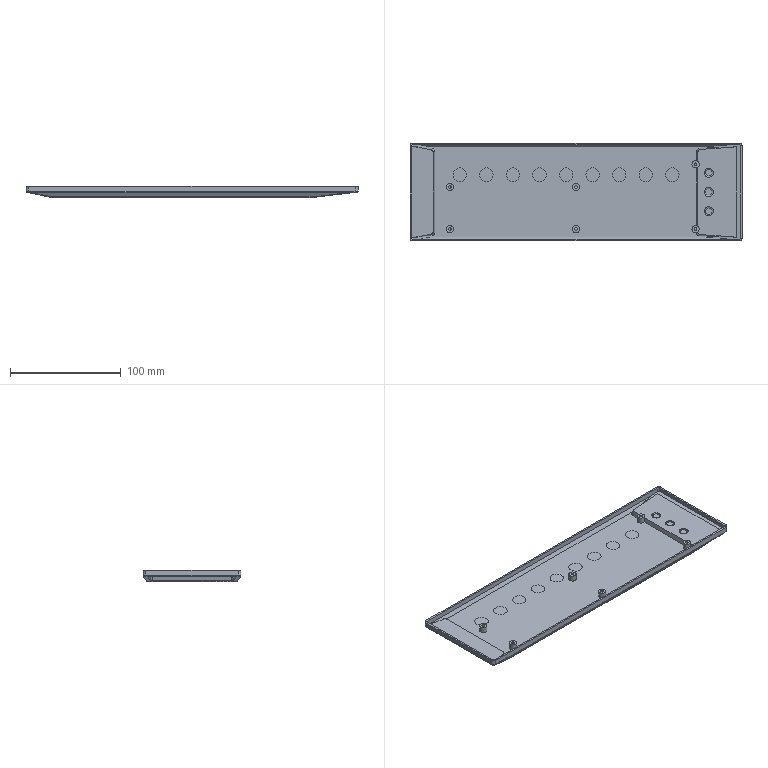NC program | NX | posted with a generic post | part box 300 x 88.5 x 10 mm
Lines 6203 to 7001 of 32249:
(CAVITY_MILL_COPY , TOOL : D4)
N12386 T04 M6
N12388 G54
N12390 G17 G0 G90 X143.356 Y-39.95 S9500 M3
N12392 G43 Z30. H4
N12394 Z0.643
N12396 G94 G1 Z-0.357 F1000.
N12398 X143.728 Y-40.393
N12400 G3 X144.494 Y-40.75 R1.
N12402 G1 X146.5 F1650.
N12404 Y-38.744
N12406 G3 X146.143 Y-37.978 R1.
N12408 G1 X145.7 Y-37.606
N12410 Z0.643
N12412 G0 Z30.
N12414 X143.356 Y-39.95
N12416 Z0.286
N12418 G1 Z-0.714 F1000.
N12420 X143.728 Y-40.393
N12422 G3 X144.494 Y-40.75 R1.
N12424 G1 X146.5 F1650.
N12426 Y-38.744
N12428 G3 X146.143 Y-37.978 R1.
N12430 G1 X145.7 Y-37.606
N12432 Z0.286
N12434 G0 X143.356 Y-39.95 Z-0.071
N12436 G1 Z-1.071 F1000.
N12438 X143.728 Y-40.393
N12440 G3 X144.494 Y-40.75 R1.
N12442 G1 X146.5 F1650.
N12444 Y-38.744
N12446 G3 X146.143 Y-37.978 R1.
N12448 G1 X145.7 Y-37.606
N12450 Z-0.071
N12452 G0 X143.356 Y-39.95 Z-0.429
N12454 G1 Z-1.429 F1000.
N12456 X143.728 Y-40.393
N12458 G3 X144.494 Y-40.75 R1.
N12460 G1 X146.5 F1650.
N12462 Y-38.744
N12464 G3 X146.143 Y-37.978 R1.
N12466 G1 X145.7 Y-37.606
N12468 Z-0.429
N12470 G0 X143.356 Y-39.95 Z-0.786
N12472 G1 Z-1.786 F1000.
N12474 X143.728 Y-40.393
N12476 G3 X144.494 Y-40.75 R1.
N12478 G1 X146.5 F1650.
N12480 Y-38.744
N12482 G3 X146.143 Y-37.978 R1.
N12484 G1 X145.7 Y-37.606
N12486 Z-0.786
N12488 G0 X143.356 Y-39.95 Z-1.143
N12490 G1 Z-2.143 F1000.
N12492 X143.728 Y-40.393
N12494 G3 X144.494 Y-40.75 R1.
N12496 G1 X146.5 F1650.
N12498 Y-38.744
N12500 G3 X146.143 Y-37.978 R1.
N12502 G1 X145.7 Y-37.606
N12504 Z-1.143
N12506 G0 X143.356 Y-39.95 Z-1.5
N12508 G1 Z-2.5 F1000.
N12510 X143.728 Y-40.393
N12512 G3 X144.494 Y-40.75 R1.
N12514 G1 X146.5 F1650.
N12516 Y-38.744
N12518 G3 X146.143 Y-37.978 R1.
N12520 G1 X145.7 Y-37.606
N12522 Z-1.5
N12524 G0 X143.356 Y-39.95 Z-1.883
N12526 G1 Z-2.883 F1000.
N12528 X143.728 Y-40.393
N12530 G3 X144.494 Y-40.75 R1.
N12532 G1 X146.5 F1650.
N12534 Y-38.744
N12536 G3 X146.143 Y-37.978 R1.
N12538 G1 X145.7 Y-37.606
N12540 Z-1.883
N12542 G0 X143.356 Y-39.95 Z-2.267
N12544 G1 Z-3.267 F1000.
N12546 X143.728 Y-40.393
N12548 G3 X144.494 Y-40.75 R1.
N12550 G1 X146.5 F1650.
N12552 Y-38.744
N12554 G3 X146.143 Y-37.978 R1.
N12556 G1 X145.7 Y-37.606
N12558 Z-2.267
N12560 G0 X143.356 Y-39.95 Z-2.65
N12562 G1 Z-3.65 F1000.
N12564 X143.728 Y-40.393
N12566 G3 X144.494 Y-40.75 R1.
N12568 G1 X146.5 F1650.
N12570 Y-38.744
N12572 G3 X146.143 Y-37.978 R1.
N12574 G1 X145.7 Y-37.606
N12576 Z-2.65
N12578 G0 X141.653 Y-39.95 Z-2.875
N12580 G1 Z-3.875 F1000.
N12582 X142.025 Y-40.393
N12584 G3 X142.791 Y-40.75 R1.
N12586 G1 X144.797 F1650.
N12588 Y-38.744
N12590 G3 X144.44 Y-37.978 R1.
N12592 G1 X143.997 Y-37.606
N12594 Z-2.875
N12596 G0 X139.848 Y-39.95 Z-3.1
N12598 G1 Z-4.1 F1000.
N12600 X140.22 Y-40.393
N12602 G3 X140.986 Y-40.75 R1.
N12604 G1 X142.992 F1650.
N12606 Y-38.744
N12608 G3 X142.635 Y-37.978 R1.
N12610 G1 X142.192 Y-37.606
N12612 Z-3.1
N12614 G0 Z30.
N12616 X118.698 Y-17.175
N12618 Z-2.6
N12620 G1 X118.679 Y-17.778 Z-2.632 F1000.
N12622 X118.955 Y-18.354 Z-2.665
N12624 X119.465 Y-18.739 Z-2.699
N12626 X119.87 Y-18.82 Z-2.72
N12628 X120. Z-2.727
N12630 X120.117 Z-2.733
N12632 X120.511 Y-18.75 Z-2.754
N12634 X121.034 Y-18.368 Z-2.788
N12636 X121.319 Y-17.786 Z-2.822
N12638 X121.301 Y-17.139 Z-2.856
N12640 X121.038 Y-16.637 Z-2.886
N12642 X120.7 Y-16.346 Z-2.909
N12644 X120.285 Y-16.181 Z-2.932
N12646 X119.719 Y-16.179 Z-2.962
N12648 X119.302 Y-16.344 Z-2.986
N12650 X118.962 Y-16.637 Z-3.009
N12652 X118.699 Y-17.139 Z-3.039
N12654 X118.679 Y-17.778 Z-3.072
N12656 X118.955 Y-18.354 Z-3.106
N12658 X119.465 Y-18.739 Z-3.139
N12660 X119.87 Y-18.82 Z-3.161
N12662 X120. Z-3.168
N12664 X120.117 Z-3.174
N12666 X120.511 Y-18.75 Z-3.195
N12668 X121.034 Y-18.368 Z-3.229
N12670 X121.319 Y-17.786 Z-3.263
N12672 X121.301 Y-17.139 Z-3.297
N12674 X121.038 Y-16.637 Z-3.326
N12676 X120.7 Y-16.346 Z-3.35
N12678 X120.285 Y-16.181 Z-3.373
N12680 X119.719 Y-16.179 Z-3.403
N12682 X119.302 Y-16.344 Z-3.426
N12684 X118.962 Y-16.637 Z-3.45
N12686 X118.699 Y-17.139 Z-3.48
N12688 X118.679 Y-17.778 Z-3.513
N12690 X118.955 Y-18.354 Z-3.547
N12692 X119.465 Y-18.739 Z-3.58
N12694 X119.87 Y-18.82 Z-3.602
N12696 X120. Z-3.609
N12698 X120.117 Z-3.615
N12700 X120.511 Y-18.75 Z-3.636
N12702 X121.034 Y-18.368 Z-3.67
N12704 X121.319 Y-17.786 Z-3.704
N12706 X121.301 Y-17.139 Z-3.737
N12708 X121.038 Y-16.637 Z-3.767
N12710 X120.7 Y-16.346 Z-3.791
N12712 X120.285 Y-16.181 Z-3.814
N12714 X119.719 Y-16.179 Z-3.844
N12716 X119.302 Y-16.344 Z-3.867
N12718 X118.962 Y-16.637 Z-3.891
N12720 X118.699 Y-17.139 Z-3.92
N12722 X118.679 Y-17.778 Z-3.954
N12724 X118.955 Y-18.354 Z-3.987
N12726 X119.465 Y-18.739 Z-4.021
N12728 X119.87 Y-18.82 Z-4.042
N12730 X120. Z-4.049
N12732 X120.117 Z-4.055
N12734 X120.511 Y-18.75 Z-4.076
N12736 X121.034 Y-18.368 Z-4.11
N12738 X121.319 Y-17.786 Z-4.144
N12740 X121.301 Y-17.139 Z-4.178
N12742 X121.038 Y-16.637 Z-4.208
N12744 X120.7 Y-16.346 Z-4.231
N12746 X120.285 Y-16.181 Z-4.255
N12748 X119.719 Y-16.179 Z-4.284
N12750 X119.302 Y-16.344 Z-4.308
N12752 X118.962 Y-16.637 Z-4.331
N12754 X118.699 Y-17.139 Z-4.361
N12756 X118.679 Y-17.778 Z-4.395
N12758 X118.955 Y-18.354 Z-4.428
N12760 X119.465 Y-18.739 Z-4.462
N12762 X119.87 Y-18.82 Z-4.483
N12764 X120. Z-4.49
N12766 G3 X121.32 Y-17.5 R1.32 F1650.
N12768 X120. Y-18.82 R-1.32
N12770 X120.766 Y-18.463 R1.
N12772 G1 Z-3.49
N12774 G0 X119.168 Y-18.231 Z-2.99
N12776 G1 X119.491 Y-18.509 Z-3.012 F1000.
N12778 X119.869 Y-18.6 Z-3.033
N12780 X120.002 Z-3.04
N12782 X120.119 Z-3.046
N12784 X120.485 Y-18.521 Z-3.065
N12786 X120.912 Y-18.167 Z-3.094
N12788 X121.12 Y-17.654 Z-3.124
N12790 X121.058 Y-17.103 Z-3.153
N12792 X120.77 Y-16.673 Z-3.18
N12794 X120.261 Y-16.401 Z-3.21
N12796 X119.744 Y-16.399 Z-3.237
N12798 X119.23 Y-16.673 Z-3.268
N12800 X118.942 Y-17.103 Z-3.295
N12802 X118.879 Y-17.645 Z-3.323
N12804 X119.078 Y-18.153 Z-3.352
N12806 X119.491 Y-18.509 Z-3.38
N12808 X119.869 Y-18.6 Z-3.401
N12810 X120.002 Z-3.408
N12812 X120.119 Z-3.414
N12814 X120.485 Y-18.521 Z-3.434
N12816 X120.912 Y-18.167 Z-3.463
N12818 X121.12 Y-17.654 Z-3.492
N12820 X121.058 Y-17.103 Z-3.521
N12822 X120.77 Y-16.673 Z-3.548
N12824 X120.261 Y-16.401 Z-3.578
N12826 X119.744 Y-16.399 Z-3.605
N12828 X119.23 Y-16.673 Z-3.636
N12830 X118.942 Y-17.103 Z-3.663
N12832 X118.879 Y-17.645 Z-3.691
N12834 X119.078 Y-18.153 Z-3.72
N12836 X119.491 Y-18.509 Z-3.748
N12838 X119.869 Y-18.6 Z-3.769
N12840 X120.002 Z-3.776
N12842 X120.119 Z-3.782
N12844 X120.485 Y-18.521 Z-3.802
N12846 X120.912 Y-18.167 Z-3.831
N12848 X121.12 Y-17.654 Z-3.86
N12850 X121.058 Y-17.103 Z-3.889
N12852 X120.77 Y-16.673 Z-3.916
N12854 X120.261 Y-16.401 Z-3.946
N12856 X119.744 Y-16.399 Z-3.973
N12858 X119.23 Y-16.673 Z-4.004
N12860 X118.942 Y-17.103 Z-4.031
N12862 X118.879 Y-17.645 Z-4.059
N12864 X119.078 Y-18.153 Z-4.088
N12866 X119.491 Y-18.509 Z-4.117
N12868 X119.869 Y-18.6 Z-4.137
N12870 X120.002 Z-4.144
N12872 X120.119 Z-4.15
N12874 X120.485 Y-18.521 Z-4.17
N12876 X120.912 Y-18.167 Z-4.199
N12878 X121.12 Y-17.654 Z-4.228
N12880 X121.058 Y-17.103 Z-4.257
N12882 X120.77 Y-16.673 Z-4.284
N12884 X120.261 Y-16.401 Z-4.314
N12886 X119.744 Y-16.399 Z-4.341
N12888 X119.23 Y-16.673 Z-4.372
N12890 X118.942 Y-17.103 Z-4.399
N12892 X118.879 Y-17.645 Z-4.428
N12894 X119.078 Y-18.153 Z-4.456
N12896 X119.491 Y-18.509 Z-4.485
N12898 X119.869 Y-18.6 Z-4.505
N12900 X120.002 Z-4.512
N12902 X120.119 Z-4.518
N12904 X120.485 Y-18.521 Z-4.538
N12906 X120.912 Y-18.167 Z-4.567
N12908 X121.12 Y-17.654 Z-4.596
N12910 X121.058 Y-17.103 Z-4.625
N12912 X120.77 Y-16.673 Z-4.652
N12914 X120.261 Y-16.401 Z-4.682
N12916 X119.744 Y-16.399 Z-4.709
N12918 X119.23 Y-16.673 Z-4.74
N12920 X118.942 Y-17.103 Z-4.767
N12922 X118.879 Y-17.645 Z-4.796
N12924 X119.078 Y-18.153 Z-4.824
N12926 X119.491 Y-18.509 Z-4.853
N12928 X119.869 Y-18.6 Z-4.873
N12930 X120. Z-4.88
N12932 X120.002 F1650.
N12934 G3 X121.1 Y-17.498 R1.1
N12936 X120. Y-18.6 R-1.1
N12938 X120.766 Y-18.243 R1.
N12940 G1 Z-3.88
N12942 G0 X119.168 Y-18.231 Z-3.38
N12944 G1 X119.491 Y-18.509 Z-3.402 F1000.
N12946 X119.869 Y-18.6 Z-3.423
N12948 X120.002 Z-3.43
N12950 X120.119 Z-3.436
N12952 X120.485 Y-18.521 Z-3.455
N12954 X120.912 Y-18.167 Z-3.484
N12956 X121.12 Y-17.653 Z-3.514
N12958 X121.058 Y-17.103 Z-3.543
N12960 X120.77 Y-16.673 Z-3.57
N12962 X120.261 Y-16.401 Z-3.6
N12964 X119.744 Y-16.399 Z-3.627
N12966 X119.23 Y-16.673 Z-3.658
N12968 X118.942 Y-17.103 Z-3.685
N12970 X118.879 Y-17.645 Z-3.713
N12972 X119.078 Y-18.153 Z-3.742
N12974 X119.491 Y-18.509 Z-3.77
N12976 X119.869 Y-18.6 Z-3.791
N12978 X120.002 Z-3.798
N12980 X120.119 Z-3.804
N12982 X120.485 Y-18.521 Z-3.824
N12984 X120.912 Y-18.167 Z-3.853
N12986 X121.12 Y-17.653 Z-3.882
N12988 X121.058 Y-17.103 Z-3.911
N12990 X120.77 Y-16.673 Z-3.938
N12992 X120.261 Y-16.401 Z-3.968
N12994 X119.744 Y-16.399 Z-3.995
N12996 X119.23 Y-16.673 Z-4.026
N12998 X118.942 Y-17.103 Z-4.053
N13000 X118.879 Y-17.645 Z-4.081
N13002 X119.078 Y-18.153 Z-4.11
N13004 X119.491 Y-18.509 Z-4.138
N13006 X119.869 Y-18.6 Z-4.159
N13008 X120.002 Z-4.166
N13010 X120.119 Z-4.172
N13012 X120.485 Y-18.521 Z-4.192
N13014 X120.912 Y-18.167 Z-4.221
N13016 X121.12 Y-17.653 Z-4.25
N13018 X121.058 Y-17.103 Z-4.279
N13020 X120.77 Y-16.673 Z-4.306
N13022 X120.261 Y-16.401 Z-4.336
N13024 X119.744 Y-16.399 Z-4.363
N13026 X119.23 Y-16.673 Z-4.394
N13028 X118.942 Y-17.103 Z-4.421
N13030 X118.879 Y-17.645 Z-4.449
N13032 X119.078 Y-18.153 Z-4.478
N13034 X119.491 Y-18.509 Z-4.507
N13036 X119.869 Y-18.6 Z-4.527
N13038 X120.002 Z-4.534
N13040 X120.119 Z-4.54
N13042 X120.485 Y-18.521 Z-4.56
N13044 X120.912 Y-18.167 Z-4.589
N13046 X121.12 Y-17.653 Z-4.618
N13048 X121.058 Y-17.103 Z-4.647
N13050 X120.77 Y-16.673 Z-4.674
N13052 X120.261 Y-16.401 Z-4.704
N13054 X119.744 Y-16.399 Z-4.731
N13056 X119.23 Y-16.673 Z-4.762
N13058 X118.942 Y-17.103 Z-4.789
N13060 X118.879 Y-17.645 Z-4.817
N13062 X119.078 Y-18.153 Z-4.846
N13064 X119.491 Y-18.509 Z-4.875
N13066 X119.869 Y-18.6 Z-4.895
N13068 X120.002 Z-4.902
N13070 X120.119 Z-4.908
N13072 X120.485 Y-18.521 Z-4.928
N13074 X120.912 Y-18.167 Z-4.957
N13076 X121.12 Y-17.653 Z-4.986
N13078 X121.058 Y-17.103 Z-5.015
N13080 X120.77 Y-16.673 Z-5.042
N13082 X120.261 Y-16.401 Z-5.072
N13084 X119.744 Y-16.399 Z-5.099
N13086 X119.23 Y-16.673 Z-5.13
N13088 X118.942 Y-17.103 Z-5.157
N13090 X118.879 Y-17.645 Z-5.186
N13092 X119.078 Y-18.153 Z-5.214
N13094 X119.491 Y-18.509 Z-5.243
N13096 X119.869 Y-18.6 Z-5.263
N13098 X120. Z-5.27
N13100 X120.002 F1650.
N13102 G3 X121.1 Y-17.498 R1.1
N13104 X120. Y-18.6 R-1.1
N13106 X120.766 Y-18.243 R1.
N13108 G1 Z-4.27
N13110 G0 X119.168 Y-18.231 Z-3.77
N13112 G1 X119.491 Y-18.509 Z-3.792 F1000.
N13114 X119.869 Y-18.6 Z-3.813
N13116 X120.002 Z-3.82
N13118 X120.119 Z-3.826
N13120 X120.485 Y-18.521 Z-3.845
N13122 X120.912 Y-18.167 Z-3.874
N13124 X121.12 Y-17.653 Z-3.904
N13126 X121.058 Y-17.103 Z-3.933
N13128 X120.77 Y-16.673 Z-3.96
N13130 X120.261 Y-16.401 Z-3.99
N13132 X119.744 Y-16.399 Z-4.017
N13134 X119.23 Y-16.673 Z-4.048
N13136 X118.942 Y-17.103 Z-4.075
N13138 X118.879 Y-17.645 Z-4.103
N13140 X119.078 Y-18.153 Z-4.132
N13142 X119.491 Y-18.509 Z-4.16
N13144 X119.869 Y-18.6 Z-4.181
N13146 X120.002 Z-4.188
N13148 X120.119 Z-4.194
N13150 X120.485 Y-18.521 Z-4.214
N13152 X120.912 Y-18.167 Z-4.243
N13154 X121.12 Y-17.653 Z-4.272
N13156 X121.058 Y-17.103 Z-4.301
N13158 X120.77 Y-16.673 Z-4.328
N13160 X120.261 Y-16.401 Z-4.358
N13162 X119.744 Y-16.399 Z-4.385
N13164 X119.23 Y-16.673 Z-4.416
N13166 X118.942 Y-17.103 Z-4.443
N13168 X118.879 Y-17.645 Z-4.471
N13170 X119.078 Y-18.153 Z-4.5
N13172 X119.491 Y-18.509 Z-4.528
N13174 X119.869 Y-18.6 Z-4.549
N13176 X120.002 Z-4.556
N13178 X120.119 Z-4.562
N13180 X120.485 Y-18.521 Z-4.582
N13182 X120.912 Y-18.167 Z-4.611
N13184 X121.12 Y-17.653 Z-4.64
N13186 X121.058 Y-17.103 Z-4.669
N13188 X120.77 Y-16.673 Z-4.696
N13190 X120.261 Y-16.401 Z-4.726
N13192 X119.744 Y-16.399 Z-4.753
N13194 X119.23 Y-16.673 Z-4.784
N13196 X118.942 Y-17.103 Z-4.811
N13198 X118.879 Y-17.645 Z-4.839
N13200 X119.078 Y-18.153 Z-4.868
N13202 X119.491 Y-18.509 Z-4.897
N13204 X119.869 Y-18.6 Z-4.917
N13206 X120.002 Z-4.924
N13208 X120.119 Z-4.93
N13210 X120.485 Y-18.521 Z-4.95
N13212 X120.912 Y-18.167 Z-4.979
N13214 X121.12 Y-17.653 Z-5.008
N13216 X121.058 Y-17.103 Z-5.037
N13218 X120.77 Y-16.673 Z-5.064
N13220 X120.261 Y-16.401 Z-5.094
N13222 X119.744 Y-16.399 Z-5.121
N13224 X119.23 Y-16.673 Z-5.152
N13226 X118.942 Y-17.103 Z-5.179
N13228 X118.879 Y-17.645 Z-5.207
N13230 X119.078 Y-18.153 Z-5.236
N13232 X119.491 Y-18.509 Z-5.265
N13234 X119.869 Y-18.6 Z-5.285
N13236 X120.002 Z-5.292
N13238 X120.119 Z-5.298
N13240 X120.485 Y-18.521 Z-5.318
N13242 X120.912 Y-18.167 Z-5.347
N13244 X121.12 Y-17.653 Z-5.376
N13246 X121.058 Y-17.103 Z-5.405
N13248 X120.77 Y-16.673 Z-5.432
N13250 X120.261 Y-16.401 Z-5.462
N13252 X119.744 Y-16.399 Z-5.489
N13254 X119.23 Y-16.673 Z-5.52
N13256 X118.942 Y-17.103 Z-5.547
N13258 X118.879 Y-17.645 Z-5.576
N13260 X119.078 Y-18.153 Z-5.604
N13262 X119.491 Y-18.509 Z-5.633
N13264 X119.869 Y-18.6 Z-5.653
N13266 X120. Z-5.66
N13268 X120.002 F1650.
N13270 G3 X121.1 Y-17.498 R1.1
N13272 X120. Y-18.6 R-1.1
N13274 X120.766 Y-18.243 R1.
N13276 G1 Z-4.66
N13278 G0 X119.168 Y-18.231 Z-4.16
N13280 G1 X119.491 Y-18.509 Z-4.182 F1000.
N13282 X119.869 Y-18.6 Z-4.203
N13284 X120.002 Z-4.21
N13286 X120.119 Z-4.216
N13288 X120.485 Y-18.521 Z-4.235
N13290 X120.912 Y-18.167 Z-4.264
N13292 X121.12 Y-17.653 Z-4.294
N13294 X121.058 Y-17.103 Z-4.323
N13296 X120.77 Y-16.673 Z-4.35
N13298 X120.261 Y-16.401 Z-4.38
N13300 X119.744 Y-16.399 Z-4.407
N13302 X119.23 Y-16.673 Z-4.438
N13304 X118.942 Y-17.103 Z-4.465
N13306 X118.879 Y-17.645 Z-4.493
N13308 X119.078 Y-18.153 Z-4.522
N13310 X119.491 Y-18.509 Z-4.55
N13312 X119.869 Y-18.6 Z-4.571
N13314 X120.002 Z-4.578
N13316 X120.119 Z-4.584
N13318 X120.485 Y-18.521 Z-4.604
N13320 X120.912 Y-18.167 Z-4.633
N13322 X121.12 Y-17.653 Z-4.662
N13324 X121.058 Y-17.103 Z-4.691
N13326 X120.77 Y-16.673 Z-4.718
N13328 X120.261 Y-16.401 Z-4.748
N13330 X119.744 Y-16.399 Z-4.775
N13332 X119.23 Y-16.673 Z-4.806
N13334 X118.942 Y-17.103 Z-4.833
N13336 X118.879 Y-17.645 Z-4.861
N13338 X119.078 Y-18.153 Z-4.89
N13340 X119.491 Y-18.509 Z-4.918
N13342 X119.869 Y-18.6 Z-4.939
N13344 X120.002 Z-4.946
N13346 X120.119 Z-4.952
N13348 X120.485 Y-18.521 Z-4.972
N13350 X120.912 Y-18.167 Z-5.001
N13352 X121.12 Y-17.653 Z-5.03
N13354 X121.058 Y-17.103 Z-5.059
N13356 X120.77 Y-16.673 Z-5.086
N13358 X120.261 Y-16.401 Z-5.116
N13360 X119.744 Y-16.399 Z-5.143
N13362 X119.23 Y-16.673 Z-5.174
N13364 X118.942 Y-17.103 Z-5.201
N13366 X118.879 Y-17.645 Z-5.229
N13368 X119.078 Y-18.153 Z-5.258
N13370 X119.491 Y-18.509 Z-5.287
N13372 X119.869 Y-18.6 Z-5.307
N13374 X120.002 Z-5.314
N13376 X120.119 Z-5.32
N13378 X120.485 Y-18.521 Z-5.34
N13380 X120.912 Y-18.167 Z-5.369
N13382 X121.12 Y-17.653 Z-5.398
N13384 X121.058 Y-17.103 Z-5.427
N13386 X120.77 Y-16.673 Z-5.454
N13388 X120.261 Y-16.401 Z-5.484
N13390 X119.744 Y-16.399 Z-5.511
N13392 X119.23 Y-16.673 Z-5.542
N13394 X118.942 Y-17.103 Z-5.569
N13396 X118.879 Y-17.645 Z-5.597
N13398 X119.078 Y-18.153 Z-5.626
N13400 X119.491 Y-18.509 Z-5.655
N13402 X119.869 Y-18.6 Z-5.675
N13404 X120.002 Z-5.682
N13406 X120.119 Z-5.688
N13408 X120.485 Y-18.521 Z-5.708
N13410 X120.912 Y-18.167 Z-5.737
N13412 X121.12 Y-17.653 Z-5.766
N13414 X121.058 Y-17.103 Z-5.795
N13416 X120.77 Y-16.673 Z-5.822
N13418 X120.261 Y-16.401 Z-5.852
N13420 X119.744 Y-16.399 Z-5.879
N13422 X119.23 Y-16.673 Z-5.91
N13424 X118.942 Y-17.103 Z-5.937
N13426 X118.879 Y-17.645 Z-5.966
N13428 X119.078 Y-18.153 Z-5.994
N13430 X119.491 Y-18.509 Z-6.023
N13432 X119.869 Y-18.6 Z-6.043
N13434 X120. Z-6.05
N13436 X120.002 F1650.
N13438 G3 X121.1 Y-17.498 R1.1
N13440 X120. Y-18.6 R-1.1
N13442 X120.766 Y-18.243 R1.
N13444 G1 Z-5.05
N13446 G0 X119.168 Y-18.231 Z-4.55
N13448 G1 X119.491 Y-18.509 Z-4.572 F1000.
N13450 X119.869 Y-18.6 Z-4.593
N13452 X120.002 Z-4.6
N13454 X120.119 Z-4.606
N13456 X120.485 Y-18.521 Z-4.625
N13458 X120.912 Y-18.167 Z-4.654
N13460 X121.12 Y-17.653 Z-4.684
N13462 X121.058 Y-17.103 Z-4.713
N13464 X120.77 Y-16.673 Z-4.74
N13466 X120.261 Y-16.401 Z-4.77
N13468 X119.744 Y-16.399 Z-4.797
N13470 X119.23 Y-16.673 Z-4.828
N13472 X118.942 Y-17.103 Z-4.855
N13474 X118.879 Y-17.645 Z-4.883
N13476 X119.078 Y-18.153 Z-4.912
N13478 X119.491 Y-18.509 Z-4.94
N13480 X119.869 Y-18.6 Z-4.961
N13482 X120.002 Z-4.968
N13484 X120.119 Z-4.974
N13486 X120.485 Y-18.521 Z-4.994
N13488 X120.912 Y-18.167 Z-5.023
N13490 X121.12 Y-17.653 Z-5.052
N13492 X121.058 Y-17.103 Z-5.081
N13494 X120.77 Y-16.673 Z-5.108
N13496 X120.261 Y-16.401 Z-5.138
N13498 X119.744 Y-16.399 Z-5.165
N13500 X119.23 Y-16.673 Z-5.196
N13502 X118.942 Y-17.103 Z-5.223
N13504 X118.879 Y-17.645 Z-5.251
N13506 X119.078 Y-18.153 Z-5.28
N13508 X119.491 Y-18.509 Z-5.308
N13510 X119.869 Y-18.6 Z-5.329
N13512 X120.002 Z-5.336
N13514 X120.119 Z-5.342
N13516 X120.485 Y-18.521 Z-5.362
N13518 X120.912 Y-18.167 Z-5.391
N13520 X121.12 Y-17.653 Z-5.42
N13522 X121.058 Y-17.103 Z-5.449
N13524 X120.77 Y-16.673 Z-5.476
N13526 X120.261 Y-16.401 Z-5.506
N13528 X119.744 Y-16.399 Z-5.533
N13530 X119.23 Y-16.673 Z-5.564
N13532 X118.942 Y-17.103 Z-5.591
N13534 X118.879 Y-17.645 Z-5.619
N13536 X119.078 Y-18.153 Z-5.648
N13538 X119.491 Y-18.509 Z-5.677
N13540 X119.869 Y-18.6 Z-5.697
N13542 X120.002 Z-5.704
N13544 X120.119 Z-5.71
N13546 X120.485 Y-18.521 Z-5.73
N13548 X120.912 Y-18.167 Z-5.759
N13550 X121.12 Y-17.653 Z-5.788
N13552 X121.058 Y-17.103 Z-5.817
N13554 X120.77 Y-16.673 Z-5.844
N13556 X120.261 Y-16.401 Z-5.874
N13558 X119.744 Y-16.399 Z-5.901
N13560 X119.23 Y-16.673 Z-5.932
N13562 X118.942 Y-17.103 Z-5.959
N13564 X118.879 Y-17.645 Z-5.987
N13566 X119.078 Y-18.153 Z-6.016
N13568 X119.491 Y-18.509 Z-6.045
N13570 X119.869 Y-18.6 Z-6.065
N13572 X120.002 Z-6.072
N13574 X120.119 Z-6.078
N13576 X120.485 Y-18.521 Z-6.098
N13578 X120.912 Y-18.167 Z-6.127
N13580 X121.12 Y-17.653 Z-6.156
N13582 X121.058 Y-17.103 Z-6.185
N13584 X120.77 Y-16.673 Z-6.212
N13586 X120.261 Y-16.401 Z-6.242
N13588 X119.744 Y-16.399 Z-6.269
N13590 X119.23 Y-16.673 Z-6.3
N13592 X118.942 Y-17.103 Z-6.327
N13594 X118.879 Y-17.645 Z-6.356
N13596 X119.078 Y-18.153 Z-6.384
N13598 X119.491 Y-18.509 Z-6.413
N13600 X119.869 Y-18.6 Z-6.433
N13602 X120. Z-6.44
N13604 X120.002 F1650.
N13606 G3 X121.1 Y-17.498 R1.1
N13608 X120. Y-18.6 R-1.1
N13610 X120.766 Y-18.243 R1.
N13612 G1 Z-5.44
N13614 G0 X119.168 Y-18.231 Z-4.94
N13616 G1 X119.491 Y-18.509 Z-4.962 F1000.
N13618 X119.869 Y-18.6 Z-4.983
N13620 X120.002 Z-4.99
N13622 X120.119 Z-4.996
N13624 X120.485 Y-18.521 Z-5.015
N13626 X120.912 Y-18.167 Z-5.044
N13628 X121.12 Y-17.653 Z-5.074
N13630 X121.058 Y-17.103 Z-5.103
N13632 X120.77 Y-16.673 Z-5.13
N13634 X120.261 Y-16.401 Z-5.16
N13636 X119.744 Y-16.399 Z-5.187
N13638 X119.23 Y-16.673 Z-5.218
N13640 X118.942 Y-17.103 Z-5.245
N13642 X118.879 Y-17.645 Z-5.273
N13644 X119.078 Y-18.153 Z-5.302
N13646 X119.491 Y-18.509 Z-5.33
N13648 X119.869 Y-18.6 Z-5.351
N13650 X120.002 Z-5.358
N13652 X120.119 Z-5.364
N13654 X120.485 Y-18.521 Z-5.384
N13656 X120.912 Y-18.167 Z-5.413
N13658 X121.12 Y-17.653 Z-5.442
N13660 X121.058 Y-17.103 Z-5.471
N13662 X120.77 Y-16.673 Z-5.498
N13664 X120.261 Y-16.401 Z-5.528
N13666 X119.744 Y-16.399 Z-5.555
N13668 X119.23 Y-16.673 Z-5.586
N13670 X118.942 Y-17.103 Z-5.613
N13672 X118.879 Y-17.645 Z-5.641
N13674 X119.078 Y-18.153 Z-5.67
N13676 X119.491 Y-18.509 Z-5.698
N13678 X119.869 Y-18.6 Z-5.719
N13680 X120.002 Z-5.726
N13682 X120.119 Z-5.732
N13684 X120.485 Y-18.521 Z-5.752
N13686 X120.912 Y-18.167 Z-5.781
N13688 X121.12 Y-17.653 Z-5.81
N13690 X121.058 Y-17.103 Z-5.839
N13692 X120.77 Y-16.673 Z-5.866
N13694 X120.261 Y-16.401 Z-5.896
N13696 X119.744 Y-16.399 Z-5.923
N13698 X119.23 Y-16.673 Z-5.954
N13700 X118.942 Y-17.103 Z-5.981
N13702 X118.879 Y-17.645 Z-6.009
N13704 X119.078 Y-18.153 Z-6.038
N13706 X119.491 Y-18.509 Z-6.067
N13708 X119.869 Y-18.6 Z-6.087
N13710 X120.002 Z-6.094
N13712 X120.119 Z-6.1
N13714 X120.485 Y-18.521 Z-6.12
N13716 X120.912 Y-18.167 Z-6.149
N13718 X121.12 Y-17.653 Z-6.178
N13720 X121.058 Y-17.103 Z-6.207
N13722 X120.77 Y-16.673 Z-6.234
N13724 X120.261 Y-16.401 Z-6.264
N13726 X119.744 Y-16.399 Z-6.291
N13728 X119.23 Y-16.673 Z-6.322
N13730 X118.942 Y-17.103 Z-6.349
N13732 X118.879 Y-17.645 Z-6.377
N13734 X119.078 Y-18.153 Z-6.406
N13736 X119.491 Y-18.509 Z-6.435
N13738 X119.869 Y-18.6 Z-6.455
N13740 X120.002 Z-6.462
N13742 X120.119 Z-6.468
N13744 X120.485 Y-18.521 Z-6.488
N13746 X120.912 Y-18.167 Z-6.517
N13748 X121.12 Y-17.653 Z-6.546
N13750 X121.058 Y-17.103 Z-6.575
N13752 X120.77 Y-16.673 Z-6.602
N13754 X120.261 Y-16.401 Z-6.632
N13756 X119.744 Y-16.399 Z-6.659
N13758 X119.23 Y-16.673 Z-6.69
N13760 X118.942 Y-17.103 Z-6.717
N13762 X118.879 Y-17.645 Z-6.746
N13764 X119.078 Y-18.153 Z-6.774
N13766 X119.491 Y-18.509 Z-6.803
N13768 X119.869 Y-18.6 Z-6.823
N13770 X120. Z-6.83
N13772 X120.002 F1650.
N13774 G3 X121.1 Y-17.498 R1.1
N13776 X120. Y-18.6 R-1.1
N13778 X120.766 Y-18.243 R1.
N13780 G1 Z-5.83
N13782 G0 X119.168 Y-18.231 Z-5.33
N13784 G1 X119.491 Y-18.509 Z-5.352 F1000.
N13786 X119.869 Y-18.6 Z-5.373
N13788 X120.002 Z-5.38
N13790 X120.119 Z-5.386
N13792 X120.485 Y-18.521 Z-5.405
N13794 X120.912 Y-18.167 Z-5.434
N13796 X121.12 Y-17.653 Z-5.464
N13798 X121.058 Y-17.103 Z-5.493
N13800 X120.77 Y-16.673 Z-5.52
N13802 X120.261 Y-16.401 Z-5.55
N13804 X119.744 Y-16.399 Z-5.577
N13806 X119.23 Y-16.673 Z-5.608
N13808 X118.942 Y-17.103 Z-5.635
N13810 X118.879 Y-17.645 Z-5.663
N13812 X119.078 Y-18.153 Z-5.692
N13814 X119.491 Y-18.509 Z-5.72
N13816 X119.869 Y-18.6 Z-5.741
N13818 X120.002 Z-5.748
N13820 X120.119 Z-5.754
N13822 X120.485 Y-18.521 Z-5.774
N13824 X120.912 Y-18.167 Z-5.803
N13826 X121.12 Y-17.653 Z-5.832
N13828 X121.058 Y-17.103 Z-5.861
N13830 X120.77 Y-16.673 Z-5.888
N13832 X120.261 Y-16.401 Z-5.918
N13834 X119.744 Y-16.399 Z-5.945
N13836 X119.23 Y-16.673 Z-5.976
N13838 X118.942 Y-17.103 Z-6.003
N13840 X118.879 Y-17.645 Z-6.031
N13842 X119.078 Y-18.153 Z-6.06
N13844 X119.491 Y-18.509 Z-6.088
N13846 X119.869 Y-18.6 Z-6.109
N13848 X120.002 Z-6.116
N13850 X120.119 Z-6.122
N13852 X120.485 Y-18.521 Z-6.142
N13854 X120.912 Y-18.167 Z-6.171
N13856 X121.12 Y-17.653 Z-6.2
N13858 X121.058 Y-17.103 Z-6.229
N13860 X120.77 Y-16.673 Z-6.256
N13862 X120.261 Y-16.401 Z-6.286
N13864 X119.744 Y-16.399 Z-6.313
N13866 X119.23 Y-16.673 Z-6.344
N13868 X118.942 Y-17.103 Z-6.371
N13870 X118.879 Y-17.645 Z-6.399
N13872 X119.078 Y-18.153 Z-6.428
N13874 X119.491 Y-18.509 Z-6.457
N13876 X119.869 Y-18.6 Z-6.477
N13878 X120.002 Z-6.484
N13880 X120.119 Z-6.49
N13882 X120.485 Y-18.521 Z-6.51
N13884 X120.912 Y-18.167 Z-6.539
N13886 X121.12 Y-17.653 Z-6.568
N13888 X121.058 Y-17.103 Z-6.597
N13890 X120.77 Y-16.673 Z-6.624
N13892 X120.261 Y-16.401 Z-6.654
N13894 X119.744 Y-16.399 Z-6.681
N13896 X119.23 Y-16.673 Z-6.712
N13898 X118.942 Y-17.103 Z-6.739
N13900 X118.879 Y-17.645 Z-6.767
N13902 X119.078 Y-18.153 Z-6.796
N13904 X119.491 Y-18.509 Z-6.825
N13906 X119.869 Y-18.6 Z-6.845
N13908 X120.002 Z-6.852
N13910 X120.119 Z-6.858
N13912 X120.485 Y-18.521 Z-6.878
N13914 X120.912 Y-18.167 Z-6.907
N13916 X121.12 Y-17.653 Z-6.936
N13918 X121.058 Y-17.103 Z-6.965
N13920 X120.77 Y-16.673 Z-6.992
N13922 X120.261 Y-16.401 Z-7.022
N13924 X119.744 Y-16.399 Z-7.049
N13926 X119.23 Y-16.673 Z-7.08
N13928 X118.942 Y-17.103 Z-7.107
N13930 X118.879 Y-17.645 Z-7.136
N13932 X119.078 Y-18.153 Z-7.164
N13934 X119.491 Y-18.509 Z-7.193
N13936 X119.869 Y-18.6 Z-7.213
N13938 X120. Z-7.22
N13940 X120.002 F1650.
N13942 G3 X121.1 Y-17.498 R1.1
N13944 X120. Y-18.6 R-1.1
N13946 X120.766 Y-18.243 R1.
N13948 G1 Z-6.22
N13950 G0 X119.168 Y-18.231 Z-5.72
N13952 G1 X119.491 Y-18.509 Z-5.742 F1000.
N13954 X119.869 Y-18.6 Z-5.763
N13956 X120.002 Z-5.77
N13958 X120.119 Z-5.776
N13960 X120.485 Y-18.521 Z-5.795
N13962 X120.912 Y-18.167 Z-5.824
N13964 X121.12 Y-17.653 Z-5.854
N13966 X121.058 Y-17.103 Z-5.883
N13968 X120.77 Y-16.673 Z-5.91
N13970 X120.261 Y-16.401 Z-5.94
N13972 X119.744 Y-16.399 Z-5.967
N13974 X119.23 Y-16.673 Z-5.998
N13976 X118.942 Y-17.103 Z-6.025